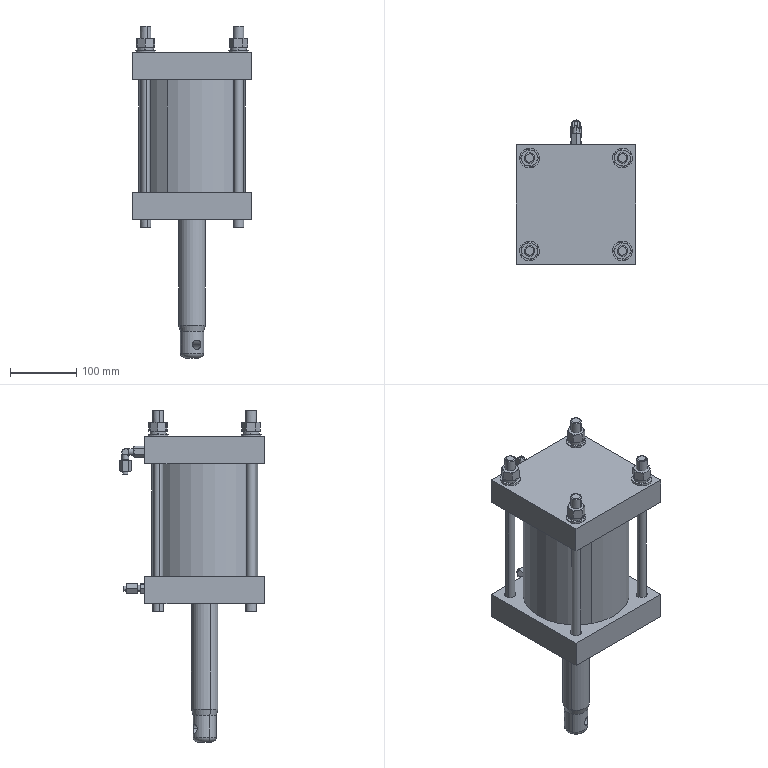Part | SolidWorks | features ReferencePattern 6, LocalCirPattern 1 | 23 solids | 549 faces | box 180 x 218.16 x 499.969 mm | volume 4201061 mm3 | cylinder 204 | cone 168 | plane 167 | torus 6 | sphere 3 | spline 1 | commonest cylinder face diameters 17 x24 16 x16 150 x16 4 x12 16.2 x12 24.356 x12